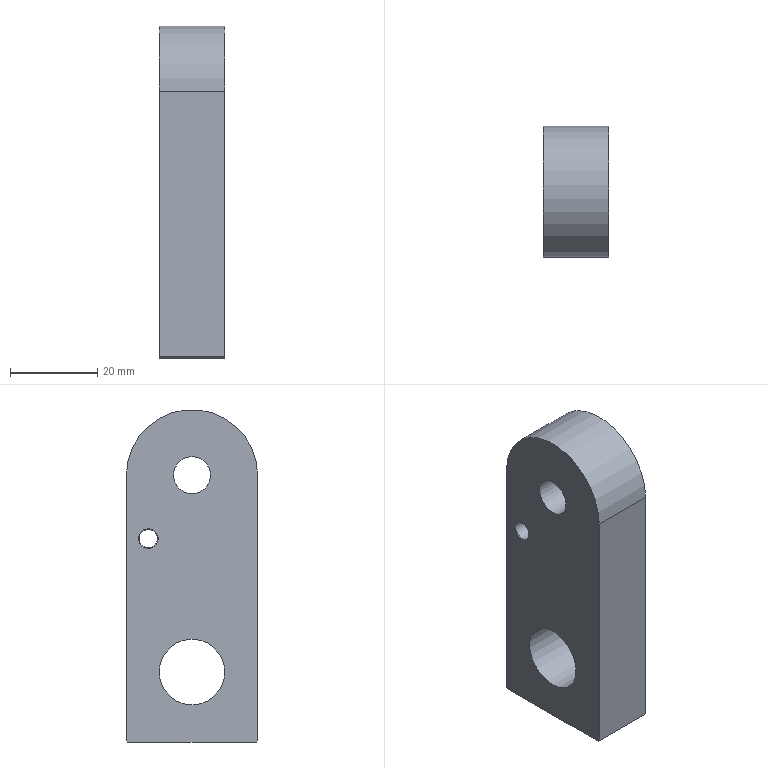NC program | NX | posted with a generic post | part box 15 x 30 x 76 mm
Lines 1 to 804 of 31310:
N10 G17 G21 G94 G90
(FLOOR_FACING_COPY_2_1 , TOOL : D63粗)
N12 T18 M6
N14 G53
N16 G17 G0 G90 X84.5 Y0. S1600 M3
N18 G43 Z50. H18
N20 Z3.1
N22 G94 G1 Z0.1 F1000.
N24 X74.5
N26 X-74.5
N28 X-84.5
N30 Z3.1
N32 G0 Z50.
N34 M5
(ADAPTIVE_MILLING , TOOL : D10.粗)
N36 T01 M6
N38 G53
N40 G17 G0 G90 X-53.524 Y0.068 S3200 M3
N42 G43 Z50. H1
N44 Z-12.5
N46 G94 G1 X-53.374 Y0.063 Z-13.437 F3000.
N48 X-53.224 Y0.057 Z-13.808
N50 X-53.075 Y0.051 Z-14.08
N52 X-52.925 Y0.045 Z-14.3
N54 X-52.775 Y0.039 Z-14.484
N56 X-52.625 Y0.034 Z-14.642
N58 X-52.475 Y0.028 Z-14.78
N60 X-52.325 Y0.022 Z-14.9
N62 X-52.175 Y0.016 Z-15.005
N64 X-52.025 Y0.011 Z-15.098
N66 X-51.875 Y0.005 Z-15.179
N68 X-51.726 Y-0.001 Z-15.25
N70 X-51.576 Y-0.007 Z-15.31
N72 X-51.426 Y-0.012 Z-15.362
N74 X-51.276 Y-0.018 Z-15.405
N76 X-51.126 Y-0.024 Z-15.439
N78 X-50.976 Y-0.03 Z-15.466
N80 X-50.826 Y-0.036 Z-15.485
N82 X-50.676 Y-0.041 Z-15.496
N84 X-50.526 Y-0.047 Z-15.5
N86 X-49.013 Y-0.105
N88 G3 X-48.002 Y0.629 R1.01
N90 X-47.708 Y3.594 R14.263
N92 X-47.639 Y16.258 R765.314
N94 G2 X-45.13 Y20.461 R5.752
N96 X-40.804 Y22.071 R9.852
N98 X-35.348 Y22.381 R41.043
N100 G1 X-28.348 Y22.4
N102 X41.297 Y22.399
N104 G2 X45.602 Y20.05 R5.632
N106 X47.289 Y15.78 R9.505
N108 X47.631 Y10.109 R39.123
N110 G1 X47.65 Y4.027
N112 X47.648 Y-16.059
N114 G2 X45.375 Y-20.277 R5.637
N116 X41.081 Y-22.026 R9.4
N118 X35.848 Y-22.375 R35.415
N120 G1 X29.286 Y-22.4
N122 X-41.303 Y-22.399
N124 G2 X-45.572 Y-20.068 R5.654
N126 X-47.282 Y-15.797 R9.474
N128 X-47.625 Y-10.607 R35.66
N130 X-47.631 Y-0.932 R525.556
N132 G3 X-47.302 Y10.662 R145.903
N134 G2 X-47.271 Y14.77 R91.878
N136 X-43.688 Y20.229 R7.103
N138 X-38.964 Y21.73 R12.267
N140 X-32.587 Y22.035 R54.418
N142 G1 X-26.769 Y22.05
N144 X39.483 Y22.049
N146 G2 X45.336 Y18.681 R7.001
N148 X46.942 Y13.998 R11.738
N150 X47.282 Y7.755 R48.352
N152 G1 X47.299 Y1.499
N154 X47.297 Y-14.289
N156 G2 X43.86 Y-20.123 R7.041
N158 X39.124 Y-21.708 R11.924
N160 X33.186 Y-22.029 R48.188
N162 G1 X25.486 Y-22.05
N164 X-39.539 Y-22.047
N166 G2 X-45.408 Y-18.554 R7.055
N168 X-46.979 Y-13.715 R12.144
N170 X-47.284 Y-7.47 R53.392
N172 X-47.07 Y2.783 R133.987
N174 G3 X-46.937 Y13.111 R379.817
N176 G2 X-42.643 Y19.894 R7.965
N178 X-37.679 Y21.369 R13.854
N180 X-30.822 Y21.685 R60.645
N182 G1 X-24.041 Y21.699
N184 X37.995 Y21.697
N186 G2 X45.187 Y17.323 R7.985
N188 X46.641 Y12.265 R14.136
N190 X46.937 Y5.362 R64.886
N192 G1 X46.949 Y-0.894
N194 G2 X46.929 Y-13.238 R899.367
N196 X42.624 Y-19.904 R7.966
N198 X37.443 Y-21.398 R14.156
N200 X31.022 Y-21.682 R62.434
N202 G1 X23.409 Y-21.699
N204 X-37.978 Y-21.697
N206 G2 X-45.19 Y-17.305 R8.
N208 X-46.631 Y-12.326 R14.078
N210 X-46.936 Y-5.468 R62.753
N212 X-46.725 Y2.807 R156.7
N214 G3 X-46.586 Y11.941 R508.028
N216 G2 X-41.635 Y19.603 R8.676
N218 X-36.341 Y21.039 R15.594
N220 X-29.176 Y21.336 R70.725
N222 G1 X-22.176 Y21.349
N224 X36.508 Y21.348
N226 G2 X41.268 Y20.244 R9.44
N228 X45.32 Y15.341 R9.325
N230 X46.406 Y9.867 R19.235
N232 X46.595 Y1.734 R122.516
N234 G1 X46.599 Y-2.597
N236 G2 X46.576 Y-12.058 R577.215
N238 X41.723 Y-19.558 R8.645
N240 X36.484 Y-21.022 R15.275
N242 X29.757 Y-21.329 R64.37
N244 G1 X22.145 Y-21.349
N246 X-36.608 Y-21.347
N248 G2 X-41.692 Y-19.982 R9.177
N250 X-45.42 Y-15.059 R9.568
N252 X-46.423 Y-9.611 R20.295
N254 X-46.423 Y1.503 R105.833
N256 G3 X-46.235 Y10.949 R566.165
N258 G2 X-43.81 Y17.084 R9.311
N260 X-38.58 Y20.086 R11.061
N262 X-32.652 Y20.885 R26.985
N264 X-21.41 Y20.999 R298.37
N266 G1 X35.252 Y20.997
N268 G2 X39.588 Y20.302 R11.523
N270 X44.628 Y15.308 R9.378
N272 X45.974 Y9.715 R17.725
N274 X46.241 Y1.541 R93.046
N276 X46.225 Y-10.934 R797.903
N278 X43.845 Y-17.042 R9.299
N280 X40.868 Y-19.233 R10.211
N282 X38.619 Y-20.22 R5.522
N284 X31.927 Y-20.917 R37.077
N286 X20.378 Y-20.999 R478.412
N288 G1 X-35.252 Y-20.997
N290 G2 X-39.627 Y-20.282 R11.493
N292 X-44.625 Y-15.303 R9.391
N294 X-45.969 Y-9.752 R17.645
N296 X-46.135 Y-0.485 R73.454
N298 G3 X-45.886 Y10.048 R831.84
N300 G2 X-44.07 Y15.669 R10.195
N302 X-38.802 Y19.411 R10.662
N304 X-32.831 Y20.467 R22.924
N306 X-23.438 Y20.645 R162.269
N308 G1 X-18.8 Y20.648
N310 X34.887 Y20.641
N312 G2 X37.704 Y20.3 R14.301
N314 X40.474 Y19.516 R5.711
N316 X43.688 Y15.882 R10.36
N318 X45.473 Y10.099 R16.373
N320 X45.87 Y3.027 R58.994
N322 X45.872 Y-9.958 R591.228
N324 X44.26 Y-15.383 R10.281
N326 X42.604 Y-17.298 R13.109
N328 X41.765 Y-18.431 R6.144
N330 X39.511 Y-19.981 R5.996
N332 X37.109 Y-20.307 R6.801
N334 X23.024 Y-20.646 R214.575
N336 G1 X19.087 Y-20.648
N338 X-33.939
N340 G2 X-38.224 Y-20.145 R14.415
N342 X-44.11 Y-14.896 R9.656
N344 X-45.56 Y-9.331 R17.456
N346 X-45.786 Y-0.941 R62.497
N348 G3 X-45.552 Y8.972 R780.203
N350 G2 X-44.258 Y14.148 R11.528
N352 X-38.829 Y18.773 R10.493
N354 X-33.034 Y20.028 R20.48
N356 X-25.341 Y20.284 R97.357
N358 G1 X-23. Y20.3
N360 X37.744 Y20.296
N362 G3 X38.512 Y20.555 R1.002
N364 G1 X38.941 Y20.948
N366 X40.405 Y22.293 Z-15.4
N368 G2 X41.331 Y22.624 R1.059 F15000.
N370 G1 X41.477 Y22.587
N372 X41.617 Y22.532
N374 X42.388 Y22.136
N376 G2 X43.149 Y21.519 R3.432
N378 G1 X43.778 Y20.834
N380 X44.4 Y20.142
N382 G2 X47.106 Y15.714 R16.299
N384 X47.814 Y13.498 R17.545
N386 X48.436 Y9.963 R26.167
N388 X48.775 Y5.018 R45.828
N390 G1 X49.001 Y-11.132
N392 G2 X48.461 Y-14.019 R7.67
N394 X47.577 Y-15.785 R10.444
N396 G1 X45.333 Y-19.371
N398 G2 X42.83 Y-21.704 R6.627
N400 G1 X41.266 Y-22.536
N402 G2 X40.135 Y-22.404 R1.
N404 G1 X38.651 Y-21.081 Z-15.5 F3000.
N406 X38.303 Y-20.766
N408 X37.943 Y-20.465
N410 G3 X37.393 Y-20.3 R1.011
N412 G1 X-25.891 Y-20.299
N414 G2 X-34.509 Y-20.26 R304.319
N416 X-40.023 Y-18.622 R10.825
N418 X-44.177 Y-13.171 R10.787
N420 X-45.319 Y-7.217 R21.978
N422 X-45.391 Y0.48 R81.442
N424 X-45.196 Y8.417 R770.408
N426 X-43.775 Y13.74 R11.87
N428 X-38.376 Y18.325 R10.798
N430 X-32.415 Y19.656 R20.666
N432 X-26.91 Y19.91 R80.646
N434 X-23.099 Y20.295 R22.208
N436 G3 X-22.347 Y21.889 R1.
N438 X-22.888 Y22.263 Z-15.466 R1.082
N440 G1 X-24.123 Y22.725 Z-15.4
N442 X-25.911 Y23.394 F15000.
N444 X-26.084 Y23.44
N446 X-26.262 Y23.457
N448 X-27.503 Y23.459
N450 X-28.744 Y23.447
N452 G3 X-31.815 Y23.089 R18.75
N454 G1 X-37.295 Y21.983
N456 G3 X-40.955 Y20.528 R11.399
N458 G1 X-41.372 Y20.26
N460 X-41.78 Y19.979
N462 X-43.792 Y18.521
N464 G3 X-45.989 Y16.106 R8.207
N466 X-46.715 Y14.63 R9.537
N468 X-47.663 Y11.694 R19.817
N470 X-48.032 Y9.562 R24.809
N472 X-48.33 Y6.791 R51.719
N474 G1 X-48.541 Y4.128
N476 X-48.737 Y1.465
N478 G3 X-48.419 Y-7.429 R47.747
N480 G1 X-48.248 Y-8.751
N482 X-48.063 Y-10.071
N484 G3 X-46.644 Y-15.204 R24.434
N486 G1 X-46.338 Y-15.977
N488 X-46.019 Y-16.743
N490 G3 X-43.811 Y-19.736 R9.327
N492 X-37.776 Y-22.832 R12.626
N494 X-34.094 Y-23.249 R21.682
N496 G1 X-26.163 Y-23.462
N498 X-25.97 Y-23.447
N500 X-25.782 Y-23.398
N502 X-24.046 Y-22.742
N504 X-22.638 Y-22.206 Z-15.476 F3000.
N506 G3 X-22.264 Y-21.912 Z-15.5 R1.011
N508 X-23. Y-20.3 R1.
N510 G2 X-26.6 Y-20.048 R70.634
N512 G3 X-33.309 Y-19.925 R287.428
N514 G2 X-38.361 Y-18.836 R12.542
N516 X-43.5 Y-13.293 R10.602
N518 X-44.894 Y-7.176 R20.007
N520 X-45.029 Y0.563 R72.419
N522 X-44.837 Y7.9 R254.973
N524 X-43.264 Y13.404 R12.11
N526 X-37.706 Y17.98 R11.177
N528 X-31.657 Y19.3 R21.547
N530 X-28.557 Y19.503 R397.476
N532 X-26.894 Y19.913 R20.739
N534 G3 X-26.107 Y21.245 R1.
N536 X-26.745 Y21.86 Z-15.454 R1.047
N538 G1 X-27.731 Y22.278 Z-15.4
N540 X-29.47 Y23.015 F15000.
N542 G3 X-30.056 Y23.075 R1.01
N544 G1 X-34.32 Y22.222
N546 G3 X-39.036 Y20.732 R22.474
N548 X-41.214 Y19.557 R18.281
N550 G1 X-42.152 Y18.968
N552 X-43.083 Y18.366
N554 G3 X-44.56 Y16.892 R6.339
N556 X-46.161 Y14.248 R21.974
N558 X-47.371 Y10.781 R11.707
N560 X-48.214 Y5.258 R85.359
N562 X-48.372 Y0.31 R28.796
N564 G1 X-47.967 Y-7.133
N566 G3 X-47.1 Y-12.632 R28.399
N568 X-44.959 Y-17.208 R12.68
N570 X-43.396 Y-18.903 R11.672
N572 G1 X-42.548 Y-19.661
N574 X-41.689 Y-20.407
N576 G3 X-39.508 Y-21.718 R9.292
N578 X-37.639 Y-22.368 R12.615
N580 X-34.607 Y-22.983 R20.402
N582 G1 X-33.991 Y-23.043
N584 X-33.373 Y-23.086
N586 X-28.447 Y-23.327
N588 G3 X-28.028 Y-23.257 R1.05
N590 G1 X-26.231 Y-22.541
N592 X-25.007 Y-22.048 Z-15.466 F3000.
N594 G3 X-24.543 Y-21.586 Z-15.5 R1.001
N596 X-25.285 Y-20.164 R1.
N598 X-30.69 Y-19.641 R28.948
N600 G2 X-35.13 Y-19.308 R26.957
N602 X-42.887 Y-13.223 R10.618
N604 X-44.453 Y-7.195 R18.713
N606 X-44.675 Y0.06 R60.469
N608 X-44.489 Y7.245 R174.076
N610 X-42.948 Y12.758 R12.662
N612 X-37.173 Y17.588 R11.416
N614 X-30.995 Y18.939 R22.025
N616 G3 X-29.913 Y19.059 R10.675
N618 G2 X-28.519 Y19.512 R8.665
N620 G3 X-27.803 Y20.73 R1.
N622 X-28.429 Y21.424 Z-15.451 R1.041
N624 G1 X-29.35 Y21.857 Z-15.4
N626 X-30.972 Y22.621 F15000.
N628 G3 X-31.682 Y22.675 R1.005
N630 G1 X-34.354 Y21.873
N632 G3 X-38.712 Y20.249 R57.868
N634 X-42.262 Y18.124 R15.962
N636 X-44.136 Y16.264 R13.095
N638 X-45.402 Y14.582 R16.376
N640 X-46.661 Y11.819 R10.128
N642 X-47.491 Y7.148 R31.229
N644 G1 X-47.69 Y5.11
N646 X-47.874 Y3.069
N648 G3 X-47.664 Y-5.822 R45.336
N650 G1 X-47.44 Y-7.671
N652 X-47.2 Y-9.518
N654 G3 X-45.541 Y-14.818 R19.53
N656 X-44.458 Y-16.849 R28.624
N658 X-41.385 Y-19.972 R9.615
N660 X-39.4 Y-21.11 R17.576
N662 X-35.156 Y-22.375 R14.229
N664 G1 X-30.391 Y-23.014
N666 G3 X-29.876 Y-22.947 R1.017
N668 G1 X-28.094 Y-22.212
N670 X-26.945 Y-21.734 Z-15.463 F3000.
N672 G3 X-26.454 Y-21.199 Z-15.5 R1.001
N674 X-27.228 Y-19.852 R1.
N676 X-30.647 Y-19.353 R14.552
N678 G2 X-34.975 Y-18.86 R25.312
N680 X-42.519 Y-12.64 R10.932
N682 X-44.096 Y-6.386 R19.303
N684 X-44.3 Y0.957 R66.105
N686 X-44.1 Y7.077 R85.025
N688 X-42.075 Y13.02 R12.252
N690 X-36.296 Y17.339 R11.99
N692 X-31.397 Y18.484 R23.856
N694 G1 X-29.903 Y19.063
N696 G3 X-29.555 Y20.717 R1.
N698 X-30.245 Y21.005 Z-15.462 R1.062
N700 G1 X-31.461 Y21.128 Z-15.4
N702 X-33.422 Y21.327 F15000.
N704 X-33.6
N706 X-33.776 Y21.299
N708 X-34.977 Y20.989
N710 X-36.174 Y20.661
N712 G3 X-42.072 Y17.382 R15.795
N714 G1 X-42.925 Y16.629
N716 X-43.766 Y15.863
N718 G3 X-44.996 Y14.239 R7.305
N720 X-46.21 Y11.534 R17.108
N722 X-46.667 Y9.615 R11.227
N724 X-47.54 Y1.956 R94.273
N726 X-47.441 Y-3.347 R33.504
N728 G1 X-47.251 Y-5.303
N730 X-47.044 Y-7.258
N732 G3 X-46.052 Y-11.896 R28.099
N734 X-44.286 Y-15.829 R18.456
N736 G1 X-43.865 Y-16.54
N738 X-43.428 Y-17.241
N740 G3 X-41.653 Y-19.046 R7.476
N742 X-39.967 Y-20.077 R11.439
N744 G1 X-38.297 Y-20.896
N746 G3 X-34.192 Y-22.219 R18.589
N748 G1 X-31.038 Y-22.844
N750 G3 X-30.434 Y-22.775 R1.008
N752 G1 X-28.774 Y-22.029
N754 X-27.667 Y-21.525 Z-15.461 F3000.
N756 G3 X-27.185 Y-20.948 Z-15.5 R1.
N758 X-27.876 Y-19.682 R1.
N760 X-31.759 Y-18.973 R18.649
N762 G2 X-36.659 Y-17.743 R15.39
N764 X-42.304 Y-11.732 R11.432
N766 X-43.756 Y-5.403 R20.661
N768 X-43.919 Y2.554 R80.223
N770 X-43.593 Y7.658 R34.906
N772 X-36.822 Y16.524 R11.488
N774 X-32.672 Y17.839 R21.311
N776 G1 X-31.259 Y18.533
N778 G3 X-30.869 Y19.983 R1.
N780 X-31.649 Y20.432 Z-15.453 R1.045
N782 G1 X-32.693 Y20.588 Z-15.4
N784 X-34.537 Y20.863 F15000.
N786 G3 X-35.132 Y20.769 R1.009
N788 G1 X-40.132 Y18.269
N790 G3 X-43.023 Y16.031 R9.432
N792 X-44.045 Y14.787 R15.631
N794 X-45.746 Y11.233 R11.637
N796 X-46.637 Y7.002 R23.982
N798 X-46.925 Y3.296 R53.974
N800 G1 X-47.012 Y1.279
N802 X-47.084 Y-0.739
N804 G3 X-46.607 Y-7.211 R36.021
N806 G1 X-46.447 Y-8.172
N808 X-46.277 Y-9.132
N810 G3 X-44.811 Y-13.677 R20.847
N812 X-42.151 Y-17.626 R15.58
N814 X-37.501 Y-20.718 R10.943
N816 G1 X-32.178 Y-22.534
N818 G3 X-31.418 Y-22.487 R1.003
N820 G1 X-29.863 Y-21.732
N822 X-28.78 Y-21.2 Z-15.461 F3000.
N824 G3 X-28.314 Y-20.6 Z-15.5 R1.
N826 X-29.016 Y-19.371 R1.
N828 X-30.733 Y-18.888 R21.875
N830 G2 X-34.687 Y-17.988 R32.211
N832 X-41.933 Y-11.194 R11.738
N834 X-43.384 Y-4.775 R21.155
N836 X-43.4 Y5.847 R73.356
N838 X-41.504 Y11.752 R13.09
N840 X-35.635 Y16.438 R12.203
N842 G1 X-33.973 Y17.049
N844 G2 X-32.631 Y17.855 R11.937
N846 G3 X-32.208 Y19.252 R1.
N848 X-32.98 Y19.751 Z-15.452 R1.043
N850 G1 X-33.997 Y19.944 Z-15.4
N852 X-35.72 Y20.272 F15000.
N854 G3 X-36.504 Y20.091 R1.002
N856 G1 X-41.483 Y16.377
N858 G3 X-44.522 Y12.643 R9.855
N860 X-46.355 Y7.393 R27.513
N862 X-46.788 Y3.107 R17.55
N864 G1 X-46.662 Y-2.482
N866 G3 X-45.766 Y-9.221 R32.027
N868 X-43.948 Y-14.335 R22.835
N870 X-41.274 Y-17.817 R12.356
N872 G1 X-40.678 Y-18.358
N874 X-40.075 Y-18.891
N876 G3 X-35.999 Y-20.869 R9.626
N878 G1 X-34.691 Y-21.157
N880 X-33.381 Y-21.433
N882 X-33.172 Y-21.434
N884 X-31.2 Y-21.239
N886 X-29.811 Y-21.096 Z-15.47 F3000.
N888 G3 X-29.288 Y-20.839 Z-15.5 R1.005
N890 X-29.611 Y-19.18 R1.
N892 X-32.872 Y-18.138 R23.804
N894 G2 X-38.345 Y-15.289 R13.471
N896 X-42.16 Y-8.98 R13.382
N898 X-43.127 Y-2.432 R27.902
N900 G1 X-43.231 Y-1.669
N902 G2 X-43.198 Y3.072 R43.121
N904 X-42.488 Y8.259 R21.018
N906 X-36.135 Y15.627 R11.85
N908 G1 X-35.548 Y15.924
N910 G2 X-33.954 Y17.061 R10.618
N912 G3 X-34.088 Y18.825 R1.
N914 X-34.738 Y18.88 Z-15.467 R1.084
N916 G1 X-36.045 Y18.669 Z-15.4
N918 X-37.878 Y18.374 F15000.
N920 G3 X-38.273 Y18.218 R1.05
N922 G1 X-38.997 Y17.738
N924 X-39.712 Y17.245
N926 G3 X-41.181 Y15.925 R10.405
N928 G1 X-41.993 Y15.047
N930 X-42.791 Y14.157
N932 G3 X-45.675 Y8.002 R13.115
N934 G1 X-46.456 Y3.649
N936 G3 X-46.399 Y3.096 R1.012
N938 G1 X-45.722 Y1.429
N940 X-45.19 Y0.129 Z-15.471 F3000.
N942 G3 X-44.803 Y-0.295 Z-15.5 R1.005
N944 X-43.294 Y0.487 R1.
N946 G1 X-43.128 Y2.638
N948 G2 X-42.519 Y6.32 R304.413
N950 X-38.674 Y13.248 R12.357
N952 X-37.509 Y14.176 R37.371
N954 X-35.53 Y15.938 R16.85
N956 G3 X-35.471 Y17.466 R1.
N958 X-36.321 Y17.716 Z-15.454 R1.047
N960 G1 X-37.39 Y17.631 Z-15.4
N962 X-39.129 Y17.492 F15000.
N964 G3 X-39.85 Y17.096 R1.002
N966 G1 X-41.015 Y15.546
N968 X-42.169 Y13.987
N970 G3 X-44.857 Y9.298 R28.294
N972 G1 X-46.186 Y6.36
N974 G3 X-46.172 Y5.505 R1.002
N976 G1 X-45.417 Y3.977
N978 X-44.869 Y2.878 Z-15.462 F3000.
N980 G3 X-44.287 Y2.42 Z-15.5 R1.001
N982 X-43.024 Y3.198 R1.
N984 G1 X-42.734 Y4.759
N986 G2 X-41.42 Y8.573 R26.782
N988 X-39.121 Y12.337 R25.033
N990 G1 X-37.782 Y13.914
N992 X-37.497 Y14.186
N994 G3 X-38.037 Y15.896 R1.
N996 X-38.676 Y15.787 Z-15.467 R1.085
N998 G1 X-39.894 Y15.257 Z-15.4
N1000 X-41.543 Y14.539 F15000.
N1002 G3 X-41.97 Y14.186 R1.013
N1004 G1 X-44.354 Y10.7
N1006 G3 X-44.515 Y9.971 R1.004
N1008 G1 X-44.226 Y8.245
N1010 X-44.123 Y7.608 Z-15.433 F3000.
N1012 X-44.008 Y6.973 Z-15.465
N1014 G3 X-43.63 Y6.405 Z-15.5 R1.001
N1016 X-42.118 Y6.827 R1.
N1018 G1 X-41.285 Y8.817
N1020 X-40.467 Y10.314
N1022 G3 X-41.377 Y11.793 R1.
N1024 X-42.024 Y11.534 Z-15.464 R1.081
N1026 G1 X-43.045 Y10.766 Z-15.4
N1028 X-44.411 Y9.74 F15000.
N1030 G3 X-44.787 Y9.157 R1.005
N1032 G1 X-45.299 Y6.855
N1034 X-45.795 Y4.55
N1036 G3 X-46.43 Y0.008 R39.842
N1038 X-46.23 Y-4.301 R18.946
N1040 G1 X-45.977 Y-5.876
N1042 X-45.708 Y-7.449
N1044 G3 X-43.956 Y-12.629 R20.632
N1046 X-41.957 Y-15.694 R16.8
N1048 G1 X-41.176 Y-16.644
N1050 X-40.372 Y-17.576
N1052 X-39.829 Y-18.157
N1054 X-39.262 Y-18.715
N1056 G3 X-37.485 Y-19.817 R6.101
N1058 G1 X-34.421 Y-21.051
N1060 G3 X-33.928 Y-21.116 R1.02
N1062 G1 X-32.081 Y-20.894
N1064 X-30.725 Y-20.726 Z-15.469 F3000.
N1066 G3 X-30.188 Y-20.436 Z-15.5 R1.003
N1068 X-30.548 Y-18.815 R1.
N1070 G2 X-34.508 Y-17.173 R247.926
N1072 X-41.503 Y-9.353 R13.039
N1074 X-42.313 Y-6.206 R22.153
N1076 G1 X-42.423 Y-5.901
N1078 X-42.94 Y-3.806
N1080 X-43.129 Y-2.419
N1082 G3 X-44.437 Y-1.606 R1.
N1084 X-45.067 Y-2.219 Z-15.454 R1.048
N1086 G1 X-45.525 Y-3.196 Z-15.4
N1088 X-46.269 Y-4.786 F15000.
N1090 G3 X-46.291 Y-5.581 R1.003
N1092 G1 X-43.754 Y-11.925
N1094 G3 X-40.92 Y-16.355 R13.825
N1096 X-39.33 Y-17.744 R12.659
N1098 G1 X-35.327 Y-20.687
N1100 G3 X-34.545 Y-20.863 R1.003
N1102 G1 X-32.852 Y-20.538
N1104 X-31.657 Y-20.303 Z-15.461 F3000.
N1106 G3 X-31.056 Y-19.853 Z-15.5 R1.
N1108 X-31.454 Y-18.451 R1.
N1110 G2 X-35.881 Y-15.944 R40.224
N1112 X-40.818 Y-9.71 R13.658
N1114 G1 X-41.688 Y-7.929
N1116 X-42.314 Y-6.201
N1118 G3 X-43.882 Y-5.764 R1.
N1120 X-44.257 Y-6.483 Z-15.458 R1.058
N1122 G1 X-44.435 Y-7.624 Z-15.4
N1124 X-44.706 Y-9.366 F15000.
N1126 G3 X-44.55 Y-10.074 R1.004
N1128 G1 X-41.436 Y-14.746
N1130 G3 X-39.013 Y-17.466 R13.101
N1132 G1 X-37.611 Y-18.656
N1134 G3 X-37.103 Y-18.883 R1.012
N1136 G1 X-35.338 Y-19.132
N1138 X-34.622 Y-19.236 Z-15.436 F3000.
N1140 X-33.905 Y-19.327 Z-15.473
N1142 G3 X-33.382 Y-19.219 Z-15.5 R1.004
N1144 X-33.291 Y-17.498 R1.
N1146 G1 X-35.09 Y-16.307
N1148 X-36.752 Y-14.932
N1150 X-38.259 Y-13.389
N1152 X-39.593 Y-11.694
N1154 G2 X-40.837 Y-9.67 R33.24
N1156 G3 X-42.661 Y-9.731 R1.
N1158 X-42.712 Y-10.345 Z-15.469 R1.094
N1160 G1 X-42.521 Y-11.694 Z-15.4
N1162 X-42.277 Y-13.423 F15000.
N1164 G3 X-41.994 Y-13.99 R1.008
N1166 G1 X-38.481 Y-17.504
N1168 G3 X-35.534 Y-19.754 R14.575
N1170 G1 X-34.992 Y-20.055
N1172 X-34.441 Y-20.339
N1174 X-33.326 Y-20.885
N1176 X-32.205 Y-21.419
N1178 G3 X-25.635 Y-23.038 R19.048
N1180 X-18.196 Y-23.345 R124.54
N1182 G1 X33.358 Y-23.841
N1184 G3 X38.278 Y-23.373 R23.76
N1186 X40.224 Y-22.894 R15.144
N1188 X45.145 Y-19.59 R11.071
N1190 X46.438 Y-17.93 R15.132
N1192 X47.892 Y-14.796 R12.374
N1194 X48.548 Y-12.144 R18.491
N1196 X48.757 Y-9.948 R19.635
N1198 X48.922 Y-4.992 R103.472
N1200 G1 X48.991 Y2.751
N1202 G3 X48.449 Y10.815 R53.486
N1204 X47.153 Y15.797 R24.873
N1206 G1 X46.115 Y18.57
N1208 G3 X45.522 Y19.158 R1.002
N1210 G1 X43.953 Y19.733
N1212 X42.66 Y20.201 Z-15.469 F3000.
N1214 G3 X42.058 Y20.189 Z-15.5 R1.004
N1216 X41.643 Y18.57 R1.
N1218 G2 X43.045 Y16.433 R6.852
N1220 X45.232 Y8.463 R22.199
N1222 X45.537 Y0.072 R93.476
N1224 X45.516 Y-9.115 R364.686
N1226 X43.253 Y-15.72 R11.273
N1228 G3 X42.901 Y-16.718 R4.233
N1230 G1 X42.531 Y-17.413
N1232 G3 X43.474 Y-18.881 R1.
N1234 X44.109 Y-18.609 Z-15.465 R1.082
N1236 G1 X45.12 Y-17.817 Z-15.4
N1238 X45.928 Y-17.184 F15000.
N1240 G3 X46.311 Y-16.401 R1.002
N1242 G1 X46.448 Y16.191
N1244 G3 X46.054 Y16.991 R1.002
N1246 G1 X45.219 Y17.628
N1248 X44.125 Y18.456 Z-15.469 F3000.
N1250 G3 X43.543 Y18.622 Z-15.5 R1.003
N1252 X42.668 Y17.204 R1.
N1254 G2 X43.236 Y15.618 R5.938
N1256 X45.067 Y5.121 R36.363
N1258 X45.163 Y-8.265 R279.426
N1260 X43.559 Y-14.27 R13.337
N1262 G3 X43.273 Y-14.977 R3.622
N1264 G2 X43.123 Y-15.981 R3.941
N1266 G3 X43.833 Y-17.238 R1.
N1268 X44.735 Y-17.031 Z-15.452 R1.042
N1270 G1 X45.573 Y-16.438 Z-15.4
N1272 X46.481 Y-15.795 F15000.
N1274 G3 X46.903 Y-14.968 R1.001
N1276 G1 X46.588 Y13.788
N1278 G3 X46.431 Y14.316 R1.013
N1280 G1 X45.751 Y15.379
N1282 X45.362 Y15.993 Z-15.437 F3000.
N1284 X44.963 Y16.6 Z-15.473
N1286 G3 X44.547 Y16.925 Z-15.5 R1.005
N1288 X43.199 Y15.744 R1.
N1290 X43.829 Y12.271 R35.993
N1292 G2 X44.77 Y2.881 R52.778
N1294 X44.832 Y-9.577 R503.6
N1296 X43.409 Y-13.678 R31.569
N1298 G3 X43.3 Y-14.701 R2.437
N1300 G1 X43.27 Y-15.006
N1302 G3 X44.471 Y-16.082 R1.
N1304 X45.145 Y-15.587 Z-15.457 R1.054
N1306 G1 X45.778 Y-14.655 Z-15.4
N1308 X46.486 Y-13.611 F15000.
N1310 G3 X46.659 Y-13.049 R1.01
N1312 G1 X46.65 Y13.292
N1314 G3 X46.476 Y13.855 R1.01
N1316 G1 X45.79 Y14.861
N1318 X45.038 Y15.956 Z-15.467 F3000.
N1320 G3 X44.495 Y16.306 Z-15.5 R1.002
N1322 X43.261 Y15.249 R1.
N1324 X43.383 Y13.398 R57.075
N1326 G2 X44.197 Y6.834 R110.153
N1328 X44.489 Y-3.835 R148.225
N1330 X44.455 Y-7.99 R73.588
N1332 X43.454 Y-12.372 R18.972
N1334 G3 X43.3 Y-12.987 R11.288
N1336 G1 Y-14.125
N1338 G3 X44.411 Y-15.119 R1.
N1340 X45.171 Y-14.626 Z-15.453 R1.044
N1342 G1 X45.778 Y-13.77 Z-15.4
N1344 X46.504 Y-12.747 F15000.
N1346 G3 X46.689 Y-12.168 R1.009
N1348 G1 Y12.444
N1350 G3 X46.504 Y13.023 R1.009
N1352 G1 X45.793 Y14.025
N1354 X45.072 Y15.032 Z-15.462 F3000.
N1356 G3 X44.437 Y15.391 Z-15.5 R1.001
N1358 X43.3 Y14.401 R1.
N1360 X43.485 Y10.496 R26.663
N1362 G2 X44.124 Y-1.948 R113.56
N1364 X44.09 Y-7.11 R85.789
N1366 X43.306 Y-11.482 R25.87
N1368 G1 X43.3 Y-12.998
N1370 G3 X44.411 Y-13.992 R1.
N1372 X45.171 Y-13.499 Z-15.453 R1.044
N1374 G1 X45.778 Y-12.643 Z-15.4
N1376 X46.504 Y-11.621 F15000.
N1378 G3 X46.689 Y-11.042 R1.009
N1380 G1 Y10.913
N1382 G3 X46.504 Y11.492 R1.009
N1384 G1 X45.793 Y12.493
N1386 X45.072 Y13.501 Z-15.462 F3000.
N1388 G3 X44.437 Y13.86 Z-15.5 R1.001
N1390 X43.3 Y12.87 R1.
N1392 X43.522 Y6.167 R71.432
N1394 G2 X43.753 Y-5.903 R168.543
N1396 X43.3 Y-9.643 R27.275
N1398 G1 Y-11.568
N1400 G3 X44.397 Y-12.564 R1.
N1402 X45.166 Y-12.078 Z-15.453 R1.044
N1404 G1 X45.778 Y-11.231 Z-15.4
N1406 X46.5 Y-10.234 F15000.
N1408 G3 X46.689 Y-9.612 R1.007
N1410 G1 X46.067 Y7.478
N1412 X46.032 Y7.705
N1414 X45.788 Y8.596
N1416 X45.263 Y10.513 Z-15.5 F3000.
N1418 G3 X43.3 Y10.245 R1.
N1420 X43.412 Y-1.94 R478.345
N1422 G2 X43.3 Y-6.687 R44.564
N1424 G1 Y-9.662
N1426 G3 X45.249 Y-9.977 R1.
N1428 G1 X45.781 Y-8.061 Z-15.4
N1430 X45.927 Y-7.548 F15000.
N1432 X46.058 Y-7.029
N1434 X46.067 Y-6.895
N1436 Y1.746
N1438 X46.056 Y1.881
N1440 X46.031 Y2.013
N1442 X45.788 Y2.888
N1444 X45.257 Y4.803 Z-15.5 F3000.
N1446 G3 X43.3 Y4.513 R1.
N1448 G1 Y-6.687
N1450 G3 X45.019 Y-7.382 R1.
N1452 X45.272 Y-6.94 Z-15.474 R1.157
N1454 G1 X45.781 Y-5.557 Z-15.4
N1456 X46.401 Y-3.869 F15000.
N1458 X46.445 Y-3.699
N1460 X46.462 Y-3.524
N1462 Y15.009
N1464 G3 X46.093 Y17.643 R9.6
N1466 G1 X45.724 Y18.934
N1468 G3 X45.097 Y19.601 R1.001
N1470 G1 X43.584 Y20.14
N1472 X42.892 Y20.388 Z-15.437 F3000.
N1474 X42.197 Y20.628 Z-15.474
N1476 G3 X41.686 Y20.635 Z-15.5 R1.006
N1478 X41.251 Y18.934 R1.
N1480 G1 X41.636 Y18.576
N1482 G3 X42.749 Y18.399 R1.011
N1484 G1 X44.379 Y19.155
N1486 X44.516 Y19.218 Z-15.496
N1488 X44.652 Y19.281 Z-15.485
N1490 X44.788 Y19.344 Z-15.466
N1492 X44.924 Y19.407 Z-15.439
N1494 X45.06 Y19.47 Z-15.405
N1496 X45.196 Y19.533 Z-15.362
N1498 X45.332 Y19.596 Z-15.31
N1500 X45.468 Y19.659 Z-15.25
N1502 X45.604 Y19.722 Z-15.179
N1504 X45.74 Y19.785 Z-15.098
N1506 X45.877 Y19.848 Z-15.005
N1508 X46.013 Y19.911 Z-14.9
N1510 X46.149 Y19.975 Z-14.78
N1512 X46.285 Y20.038 Z-14.642
N1514 X46.421 Y20.101 Z-14.484
N1516 X46.557 Y20.164 Z-14.3
N1518 X46.693 Y20.227 Z-14.08
N1520 X46.829 Y20.29 Z-13.808
N1522 X46.965 Y20.353 Z-13.437
N1524 X47.101 Y20.416 Z-12.5
N1526 G0 Z50.
N1528 M5
(DRILLING , TOOL : D8点钻)
N1530 T03 M6
N1532 G53
N1534 G17 G0 G90 X-23. Y0. S1500 M3
N1536 G43 Z50. H3
N1538 G94 G81 G98 Z-2.7 F100. R3.
N1540 X22.
N1542 X-8.5 Y10.
N1544 G80
N1546 G0 X-8.5 Y10. Z50.
N1548 M5
(PECK_DRILLING , TOOL : Z8.5)
N1550 T04 M6
N1552 G53
N1554 G17 G0 G90 X-23. Y0. S1200 M3
N1556 G43 Z50. H4
N1558 G94 G83 G99 Z-22. F80. Q2. R3.
N1560 X22.
N1562 G80
N1564 G0 X22. Y0. Z50.
N1566 M5
(PECK_DRILLING_COPY_1 , TOOL : Z4.2)
N1568 T14 M6
N1570 G53
N1572 G17 G0 G90 X-8.5 Y10. S1200 M3
N1574 G43 Z50. H14
N1576 G94 G83 G99 Z-20. F80. Q2. R3.
N1578 G80
N1580 G0 X-8.5 Y10. Z50.
N1582 M5